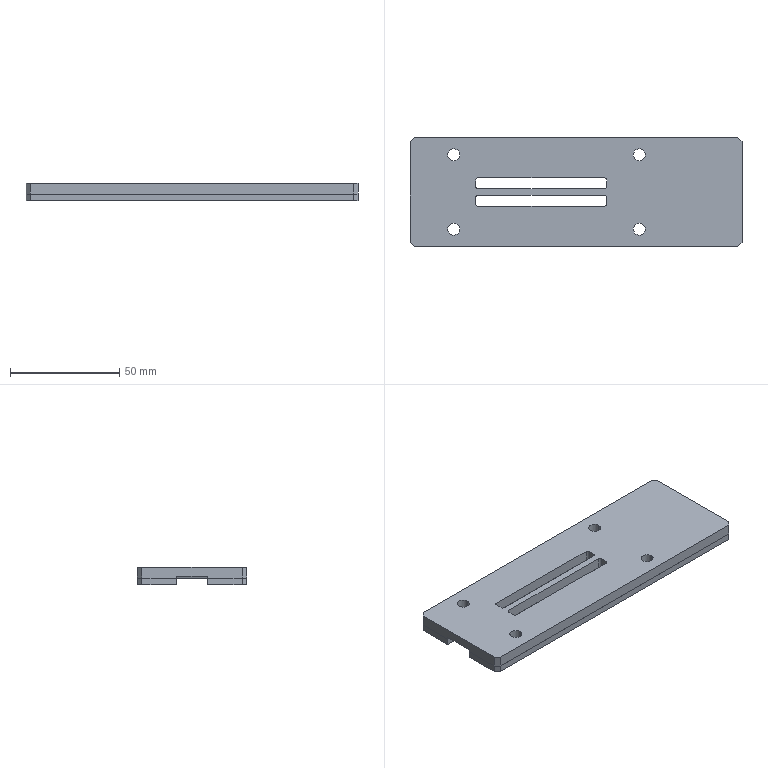Part | STEP file | PN_0019 Mount electronic clip transparent acrylic cover plate | 1 solid | 61 faces | box 152 x 50 x 8 mm | volume 50516 mm3 | plane 45 | cylinder 16 | commonest cylinder face diameters 2 x8 5.5 x8